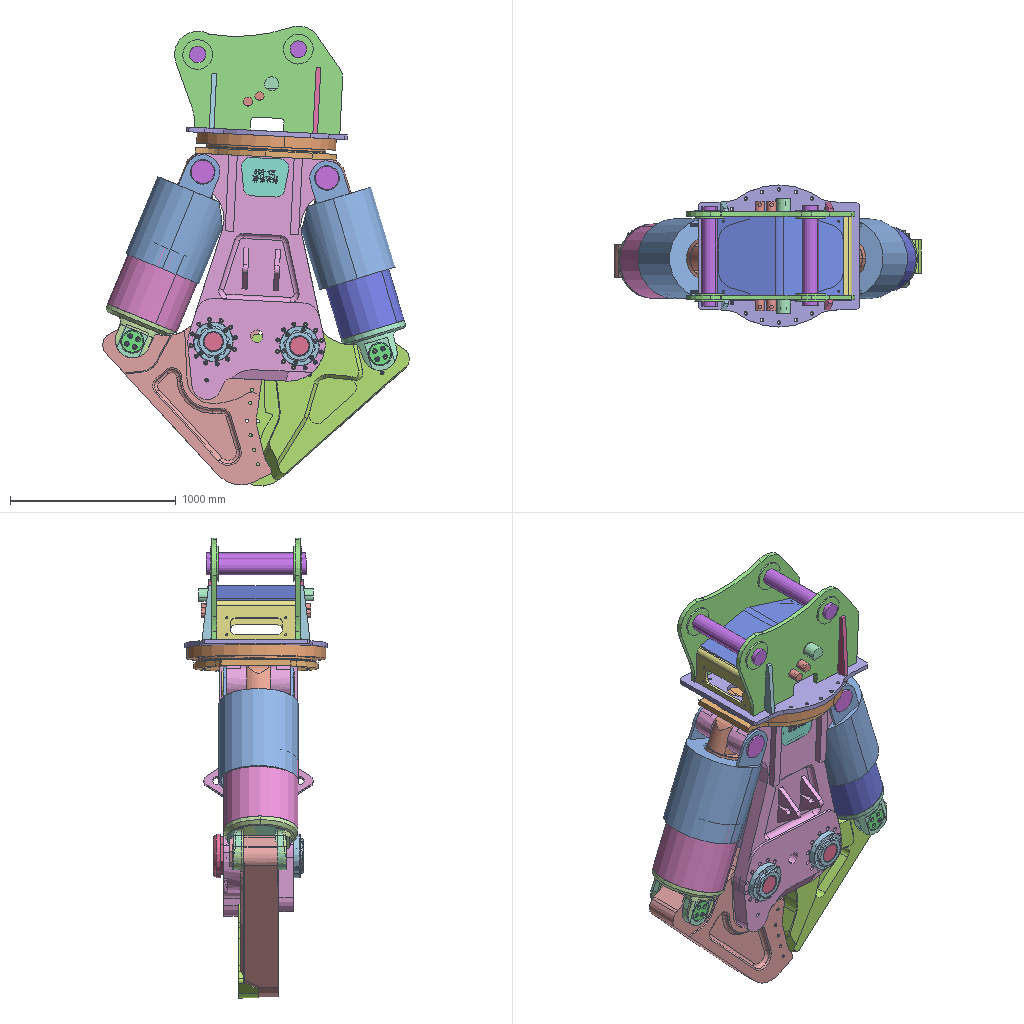Assembly | SolidWorks | 36 different items | 73 placed | box 1847 x 857 x 2773 mm
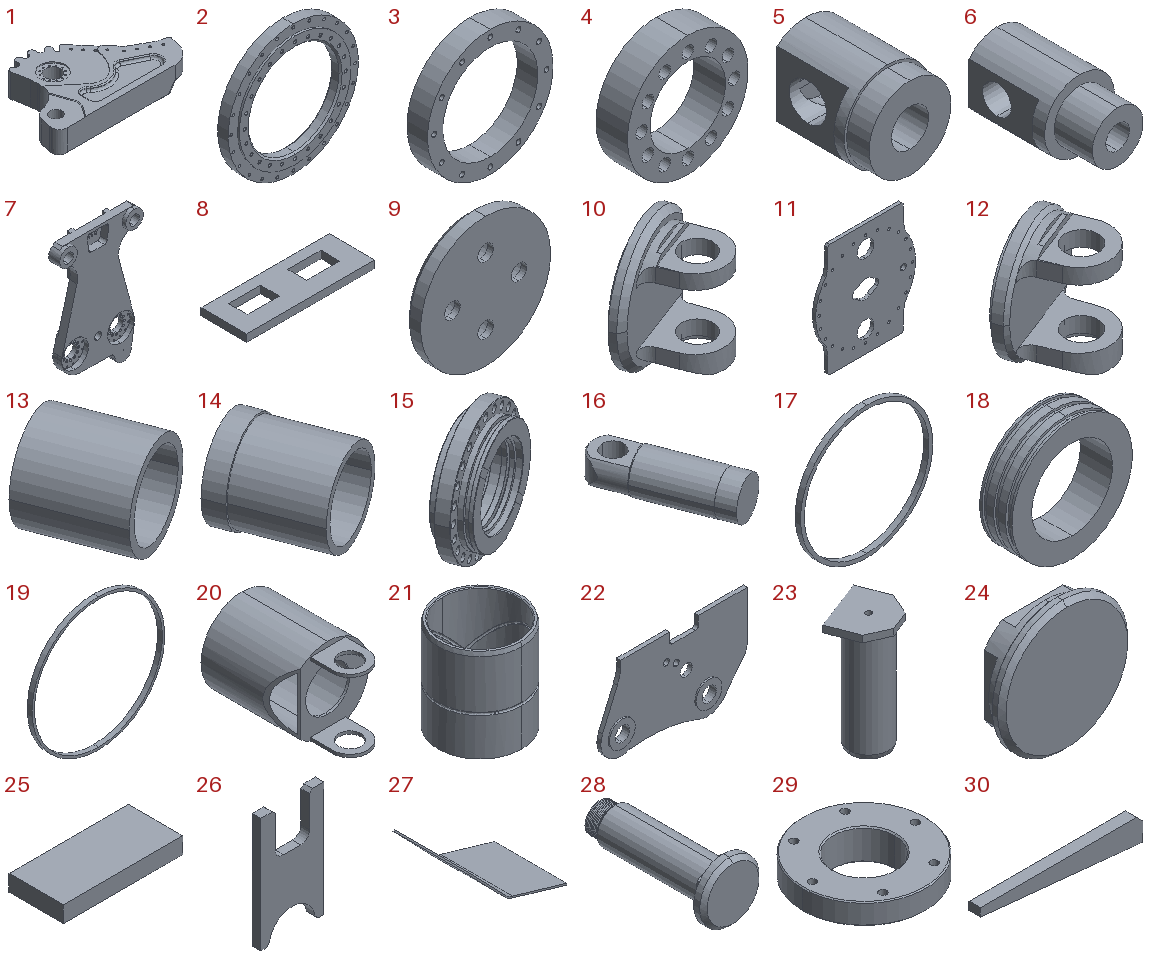Parts list (item | quantity | size | volume | features):
1 | x1 | 1278 x 806.277 x 230 mm | 104700770 mm3 | features ICE 6, MoveFace 5, BaseBody 2, Chamfer 1, HoleWzd 1
2 | x1 | 840 x 80 x 840 mm | 18083089 mm3 | features ICE 3, HoleWzd 2, Chamfer 1, Extrusion 1
3 | x4 | 304 x 50 x 304 mm | 1483680 mm3 | features HoleWzd 2, ICE 2, Extrusion 1
4 | x4 | 230 x 60 x 230 mm | 1319398 mm3 | features Extrusion 1, ICE 1
5 | x2 | 85 x 102 x 85 mm | 399159 mm3 | features ICE 4, Extrusion 1
6 | x4 | 55 x 95 x 55 mm | 152228 mm3 | features ICE 4, Extrusion 1
7 | x2 | 949.998 x 259.953 x 1480 mm | 71064561 mm3 | features ICE 19, Fillet 4, HoleWzd 2, Extrusion 1, SweepCut 1
8 | x1 | 616 x 220 x 35 mm | 3748166 mm3 | features Extrusion 1, ICE 1
9 | x2 | 140.4 x 18 x 140.4 mm | 234372 mm3 | features BaseBody 1, Scale 1
10 | x1 | 420.674 x 323.225 x 450 mm | 11948863 mm3 | features ICE 3, MoveFace 2, BaseBody 1, Chamfer 1, Scale 1
11 | x1 | 857 x 28 x 970 mm | 18025992 mm3 | features Extrusion 1, ICE 1
12 | x2 | 381.228 x 317.121 x 396 mm | 10472227 mm3 | features MoveFace 2, BaseBody 1, Scale 1
13 | x1 | 580.701 x 579.323 x 450 mm | 23061301 mm3 | features ICE 2, BaseBody 1, Scale 1
14 | x2 | 538.702 x 563.166 x 414 mm | 15927299 mm3 | features BaseBody 1, Scale 1
15 | x2 | 400.613 x 225.724 x 414 mm | 6404045 mm3 | features BaseBody 1, Scale 1
16 | x2 | 436.641 x 719.533 x 228 mm | 24273606 mm3 | features MoveFace 2, BaseBody 1, Scale 1
17 | x2 | 336 x 13.8 x 336 mm | 135847 mm3 | features BaseBody 1, Scale 1
18 | x2 | 336 x 90 x 336 mm | 4158634 mm3 | features BaseBody 1, Scale 1
19 | x6 | 336 x 12 x 336 mm | 74644 mm3 | features BaseBody 1, Scale 1
20 | x2 | 481 x 737 x 481 mm | 11479821 mm3 | features ICE 3, MoveFace 3, BaseBody 1, Scale 1
21 | x2 | 126 x 126 x 140 mm | 308538 mm3 | features BaseBody 1, ICE 1, Scale 1
22 | x2 | 1020 x 48 x 641.98 mm | 14814063 mm3 | features ICE 2, Extrusion 1
23 | x2 | 177.912 x 167.575 x 330 mm | 3479602 mm3 | features BaseBody 1, Scale 1
24 | x2 | 150 x 40 x 150 mm | 549544 mm3 | features ICE 3, Chamfer 2, BaseBody 1
25 | x2 | 220 x 100 x 30 mm | 660000 mm3 | features Extrusion 1
26 | x2 | 220 x 30 x 400 mm | 1803857 mm3 | features Chamfer 1, Extrusion 1, Fillet 1
27 | x1 | 669.894 x 475 x 409.47 mm | 3812408 mm3 | features Extrusion 1, Fillet 1
28 | x2 | 240 x 540 x 240 mm | 9830970 mm3 | features ICE 4, Chamfer 2, Extrusion 1, Helix 1, SweepCut 1
29 | x2 | 240 x 240 x 60 mm | 1562798 mm3 | features ICE 3, BaseBody 1, Chamfer 1, Scale 1
30 | x2 | 400 x 28 x 60 mm | 444850 mm3 | features Extrusion 1
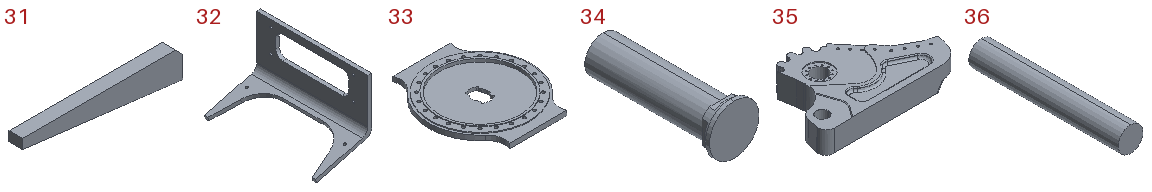31 | x2 | 330 x 28 x 60 mm | 366450 mm3 | features Extrusion 1
32 | x2 | 241.053 x 478 x 290.926 mm | 1872027 mm3 | features HoleWzd 2, ICE 2, Extrusion 1
33 | x1 | 750 x 850 x 47 mm | 14896287 mm3 | features ICE 4, BaseBody 1
34 | x2 | 150 x 396 x 150 mm | 3942504 mm3 | features ICE 4, BaseBody 1
35 | x1 | 1278 x 813.2 x 230 mm | 107497671 mm3 | features ICE 7, MoveFace 5, BaseBody 2, Chamfer 1, HoleWzd 1
36 | x2 | 100 x 600 x 100 mm | 4712389 mm3 | features Extrusion 1
Mates (type | each side: item.copy, entity, surface, feature):
Coincident | 1.1 face plane Input 1 | 7.1 face plane Boss-Extrude1
Coincident | 35.1 face plane Input 2 | 7.1 face plane Boss-Extrude1
Coincident | 35.1 face plane Input 1 | 7.2 face plane Boss-Extrude1
Coincident | 7.2 face plane Boss-Extrude1 | 33.1 face plane Input 1
Coincident | 7.2 edge | 33.1 select_type:24
Coincident | 7.2 vertex | 33.1 select_type:25
Coincident | 7.1 face plane Boss-Extrude1 | 26.1 face plane Boss-Extrude1 | 2 times
Coincident | 7.2 face plane Boss-Extrude1 | 26.2 face plane Boss-Extrude1 | 2 times
Parallel | 26.1 edge | 26.2 edge
DistanceDim | 26.2 vertex | 33.1 face plane Input 1
Coincident | 33.1 face plane Input 1 | 25.1 face plane Boss-Extrude1
Coincident | 7.2 face plane Boss-Extrude1 | 25.1 face plane Boss-Extrude1
Tangent | 7.2 face cylinder Boss-Extrude1 | 25.1 face plane Boss-Extrude1
Coincident | 33.1 face plane Input 1 | 25.2 face plane Boss-Extrude1
Coincident | 7.1 face plane Boss-Extrude1 | 25.2 face plane Boss-Extrude1
Tangent | 7.1 face cylinder Boss-Extrude1 | 25.2 face plane Boss-Extrude1
Coincident | 7.1 face plane Boss-Extrude1 | 28.1 face plane Boss-Extrude1
Concentric | 28.1 edge | 29.1 face cylinder Input 1
Coincident | 7.2 face plane Boss-Extrude1 | 29.1 face plane Input 1
Concentric | 29.2 face cylinder Input 1 | 28.2 edge
Coincident | 7.1 face plane Boss-Extrude1 | 28.2 face plane Boss-Extrude1
Coincident | 7.2 face plane Boss-Extrude1 | 29.2 face plane Input 1
Coincident | 7.1 face plane Cut-Extrude2 | 34.1 face plane Input 1
Parallel | 7.2 face plane Cut-Extrude6 | 24.1 face plane Boss-Extrude3
Coincident | 7.2 face plane Cut-Extrude2 | 24.1 face plane Input 1
Coincident | 7.1 face plane Cut-Extrude2 | 34.2 face plane Input 1
Parallel | 7.2 face plane Cut-Extrude6 | 24.2 face plane Boss-Extrude3
Coincident | 7.2 face plane Cut-Extrude2 | 24.2 face plane Input 1
Concentric | 12.1 face cylinder Input 1 | 14.1 face cylinder Input 1
Coincident | 12.1 face plane Input 1 | 14.1 face plane Input 1
Concentric | 16.1 face cylinder Input 1 | 18.1 face cylinder Input 1
Coincident | 16.1 face plane Input 1 | 18.1 face plane Input 1
Concentric | 16.1 face cylinder Input 1 | 21.1 face cylinder Input 1
Coincident | 16.1 face plane Input 1 | 21.1 face plane Cut-Extrude1
Coincident | 7.2 face plane Boss-Extrude5 | 16.1 face plane Input 1
Concentric | 16.1 face cylinder Input 1 | 15.1 face cylinder Input 1
Concentric | 15.1 face cylinder Input 1 | 17.1 face cylinder Input 1
Coincident | 15.1 face plane Input 1 | 17.1 face plane Input 1
Coincident | 18.1 face cylinder Input 1 | 19.1 edge
Coincident | 18.1 face plane Input 1 | 19.1 face plane Input 1
Concentric | 18.1 face cylinder Input 1 | 19.2 face cylinder Input 1
Concentric | 18.1 face cylinder Input 1 | 19.3 face cylinder Input 1
Coincident | 18.1 face plane Input 1 | 19.3 face plane Input 1
Coincident | 18.1 face plane Input 1 | 19.2 face plane Input 1
Concentric | 16.1 face cylinder Input 1 | 14.1 face cylinder Input 1
Coincident | 14.1 face plane Input 1 | 15.1 face plane Input 1
Concentric | 35.1 face cylinder Boss-Extrude2 | 12.1 face cylinder Input 1
Parallel | 35.1 face plane Input 1 | 12.1 face plane Input 1
Coincident | 18.2 face plane Input 1 | 16.2 face plane Input 1
Coincident | 21.2 face plane Cut-Extrude1 | 16.2 face plane Input 1
Coincident | 19.4 face plane Input 1 | 18.2 face plane Input 1
Coincident | 15.2 face plane Input 1 | 14.2 face plane Input 1
Coincident | 19.5 face plane Input 1 | 18.2 face plane Input 1
Coincident | 19.5 edge | 18.2 face cylinder Input 1
Coincident | 17.2 face plane Input 1 | 15.2 face plane Input 1
Coincident | 19.6 face plane Input 1 | 18.2 face plane Input 1
Coincident | 12.2 face plane Input 1 | 14.2 face plane Input 1
Concentric | 17.2 face cylinder Input 1 | 15.2 face cylinder Input 1
Concentric | 14.2 face cylinder Input 1 | 16.2 face cylinder Input 1
Concentric | 18.2 face cylinder Input 1 | 16.2 face cylinder Input 1
Concentric | 15.2 face cylinder Input 1 | 16.2 face cylinder Input 1
Concentric | 12.2 face cylinder Input 1 | 14.2 face cylinder Input 1
Concentric | 21.2 face cylinder Input 1 | 16.2 face cylinder Input 1
Concentric | 19.6 face cylinder Input 1 | 18.2 face cylinder Input 1
Concentric | 19.4 face cylinder Input 1 | 18.2 face cylinder Input 1
Coincident | 7.2 face plane Boss-Extrude5 | 16.2 face plane Input 1
Concentric | 1.1 face cylinder Boss-Extrude2 | 12.2 face cylinder Input 1
Concentric | 12.1 face cylinder Input 1 | 9.1 face cylinder Input 1
Coincident | 12.1 face plane Input 1 | 9.1 face plane Input 1
Concentric | 12.2 face cylinder Input 1 | 9.2 face cylinder Input 1
Coincident | 12.2 face plane Input 1 | 9.2 face plane Input 1
Concentric | 34.1 edge | 24.1 face cylinder Boss-Extrude2
Concentric | 7.1 face cylinder Cut-Extrude5 | 34.1 face cylinder Boss-Extrude4
Concentric | 7.2 face cylinder Cut-Extrude5 | 34.2 face cylinder Boss-Extrude4
Concentric | 34.2 edge | 24.2 face cylinder Boss-Extrude1
Concentric | 12.2 face cylinder Input 1 | 23.1 face cylinder Input 1
Coincident | 12.2 face plane Input 1 | 23.1 face plane Input 1 | 2 times
Concentric | 12.1 face cylinder Input 1 | 23.2 face cylinder Input 1
Coincident | 12.1 face plane Input 1 | 23.2 face plane Input 1 | 2 times
Concentric | 34.1 face cylinder Boss-Extrude4 | 21.1 edge
Concentric | 34.2 face cylinder Boss-Extrude4 | 21.2 edge
Concentric | 24.1 face cylinder Boss-Extrude2 | 20.1 face cylinder Boss-Extrude2
Coincident | 7.2 face plane Cut-Extrude2 | 20.1 face plane Input 1
Concentric | 14.1 face cylinder Input 1 | 20.1 face cylinder Input 1
Concentric | 24.2 face cylinder Boss-Extrude2 | 20.2 face cylinder Boss-Extrude1
Coincident | 7.2 face plane Cut-Extrude2 | 20.2 face plane Input 1
Concentric | 14.2 face cylinder Input 1 | 20.2 face cylinder Input 1
Concentric | 7.2 face cylinder Cut-Extrude7 | 3.1 face cylinder Boss-Extrude1
Coincident | 7.2 face plane Cut-Extrude7 | 3.1 face plane Boss-Extrude1
Concentric | 7.1 face cylinder Cut-Extrude7 | 3.2 face cylinder Boss-Extrude1
Coincident | 7.1 face plane Cut-Extrude7 | 3.2 face plane Boss-Extrude1
Concentric | 7.1 face cylinder Cut-Extrude7 | 3.3 face cylinder Boss-Extrude1
Coincident | 7.1 face plane Cut-Extrude7 | 3.3 face plane Boss-Extrude1
Concentric | 7.2 face cylinder Cut-Extrude7 | 3.4 face cylinder Boss-Extrude1
Coincident | 7.2 face plane Cut-Extrude7 | 3.4 face plane Boss-Extrude1
Concentric | 7.1 face cylinder Boss-Extrude6 | 28.2 face cylinder Boss-Extrude2
Concentric | 7.1 face cylinder Boss-Extrude6 | 28.1 face cylinder Boss-Extrude2
Concentric | 7.1 face cylinder Boss-Extrude6 | 3.1 face cylinder Cut-Extrude1
Concentric | 7.1 face cylinder Boss-Extrude6 | 3.4 face cylinder Cut-Extrude1
Concentric | 9.1 face cylinder Input 1 | 23.2 face cylinder Input 1
Concentric | 9.2 face cylinder Input 1 | 23.1 face cylinder Input 1
Concentric | 7.2 face cylinder Cut-Extrude8 | 3.4 face cylinder M14 Tapped Hole1
Concentric | 7.2 face cylinder Cut-Extrude8 | 3.1 face cylinder M14 Tapped Hole1
Concentric | 7.1 face cylinder Cut-Extrude8 | 3.3 face cylinder M14 Tapped Hole1
Concentric | 7.1 face cylinder Cut-Extrude8 | 3.2 face cylinder M14 Tapped Hole1
Concentric | 35.1 face cylinder Boss-Extrude3 | 28.1 face cylinder Boss-Extrude2
Concentric | 1.1 face cylinder Boss-Extrude3 | 28.2 face cylinder Boss-Extrude2
Concentric | 7.2 face cylinder M14 Tapped Hole1 | 29.1 face cylinder Boss-Extrude1
Concentric | 28.1 face cylinder Boss-Extrude2 | 4.1 face cylinder Boss-Extrude1
Concentric | 35.1 face cylinder M14 Tapped Hole1 | 4.1 face cylinder Cut-Extrude1
Coincident | 35.1 face plane Input 1 | 4.1 face plane Boss-Extrude1
Concentric | 3.1 face cylinder Cut-Extrude1 | 4.2 face cylinder Boss-Extrude1
Coincident | 1.1 face plane Cut-Extrude3 | 4.2 face plane Boss-Extrude1
Concentric | 1.1 face cylinder M14 Tapped Hole1 | 4.2 face cylinder Cut-Extrude1
Concentric | 3.2 face cylinder Cut-Extrude1 | 4.3 face cylinder Boss-Extrude1
Coincident | 1.1 face plane Cut-Extrude4 | 4.3 face plane Boss-Extrude1
Concentric | 1.1 face cylinder M14 Tapped Hole1 | 4.3 face cylinder Cut-Extrude1
Concentric | 3.3 face cylinder Cut-Extrude1 | 4.4 face cylinder Boss-Extrude1
Concentric | 35.1 edge | 4.4 face cylinder Boss-Extrude1
Coincident | 35.1 face plane Cut-Extrude4 | 4.4 face plane Boss-Extrude1
GearDim | 35.1 select_type:24 | 1.1 select_type:24
Coincident | 7.2 face plane Boss-Extrude1 | 8.1 face plane Boss-Extrude1
Parallel | 7.2 face plane Boss-Extrude1 | 8.1 face plane Boss-Extrude1
DistanceDim | 7.2 face plane Boss-Extrude1 | 8.1 face plane Boss-Extrude1
Concentric | 33.1 face cylinder Input 1 | 2.1 face cylinder Boss-Extrude1
Coincident | 33.1 face plane Input 1 | 2.1 face plane Boss-Extrude2
Concentric | 33.1 face cylinder Cut-Extrude2 | 2.1 face cylinder M20 Tapped Hole2
Coincident | 2.1 face plane Boss-Extrude1 | 11.1 face plane Boss-Extrude1
Concentric | 2.1 face cylinder Boss-Extrude1 | 11.1 face cylinder Boss-Extrude1
Concentric | 2.1 face cylinder M20 Tapped Hole1 | 11.1 face cylinder Cut-Extrude1
Coincident | 11.1 face plane Boss-Extrude1 | 22.1 face plane Boss-Extrude1 | 2 times
Coincident | 11.1 select_type:24 | 22.1 edge | 2 times
Coincident | 11.1 face plane Boss-Extrude1 | 22.2 face plane Boss-Extrude1
Coincident | 11.1 select_type:24 | 22.2 edge | 2 times
Coincident | 11.1 face plane Boss-Extrude1 | 30.1 face plane Boss-Extrude1
Coincident | 22.2 face plane Boss-Extrude1 | 30.1 face plane Boss-Extrude1
Coincident | 11.1 face plane Boss-Extrude1 | 31.1 face plane Boss-Extrude1
Coincident | 22.2 face plane Boss-Extrude1 | 31.1 face plane Boss-Extrude1
Coincident | 11.1 face plane Boss-Extrude1 | 30.2 face plane Boss-Extrude1
Coincident | 22.1 face plane Boss-Extrude1 | 30.2 face plane Boss-Extrude1
Coincident | 11.1 face plane Boss-Extrude1 | 31.2 face plane Boss-Extrude1
Coincident | 22.1 face plane Boss-Extrude1 | 31.2 face plane Boss-Extrude1
Coincident | 11.1 face plane Boss-Extrude1 | 32.1 face plane Boss-Extrude1
Coincident | 11.1 select_type:24 | 32.1 edge
Coincident | 22.1 face plane Boss-Extrude1 | 32.1 face plane Boss-Extrude1
Coincident | 11.1 face plane Boss-Extrude1 | 32.2 face plane Boss-Extrude1
Coincident | 11.1 select_type:24 | 32.2 edge
Coincident | 22.1 face plane Boss-Extrude1 | 32.2 face plane Boss-Extrude1
Concentric | 22.2 face cylinder Boss-Extrude2 | 36.1 face cylinder Boss-Extrude1
Concentric | 22.2 face cylinder Boss-Extrude2 | 36.2 face cylinder Boss-Extrude1
Concentric | 22.2 face cylinder Boss-Extrude1 | 5.1 face cylinder Boss-Extrude1
Coincident | 22.2 face plane Boss-Extrude1 | 5.1 edge
Concentric | 22.1 face cylinder Boss-Extrude1 | 5.2 face cylinder Boss-Extrude1
Coincident | 22.1 face plane Boss-Extrude1 | 5.2 edge
Concentric | 22.1 edge | 6.1 face cylinder Boss-Extrude1
Coincident | 22.1 face plane Boss-Extrude1 | 6.1 face plane Boss-Extrude2
Concentric | 22.1 face cylinder Boss-Extrude1 | 6.2 face cylinder Boss-Extrude1
Coincident | 22.1 face plane Boss-Extrude1 | 6.2 face plane Boss-Extrude2
Concentric | 22.2 face cylinder Boss-Extrude1 | 6.3 face cylinder Boss-Extrude1
Coincident | 22.2 face plane Boss-Extrude1 | 6.3 face plane Boss-Extrude2
Concentric | 22.2 face cylinder Boss-Extrude1 | 6.4 face cylinder Boss-Extrude1
Coincident | 22.2 face plane Boss-Extrude1 | 6.4 face plane Boss-Extrude2
Coincident | 32.2 face plane Boss-Extrude1 | 27.1 face plane Boss-Extrude1
Coincident | 22.1 face plane Boss-Extrude1 | 27.1 face plane Boss-Extrude1
Concentric | 10.1 face cylinder Boss-Extrude1 | 13.1 face cylinder Boss-Extrude1
Coincident | 10.1 face plane Input 1 | 13.1 face plane Input 1
Concentric | 12.1 face cylinder Input 1 | 10.1 face cylinder Input 1
Coincident | 35.1 face plane Input 1 | 10.1 face plane Input 1
Parallel | 20.1 face cylinder Input 1 | 13.1 face cylinder Boss-Extrude1